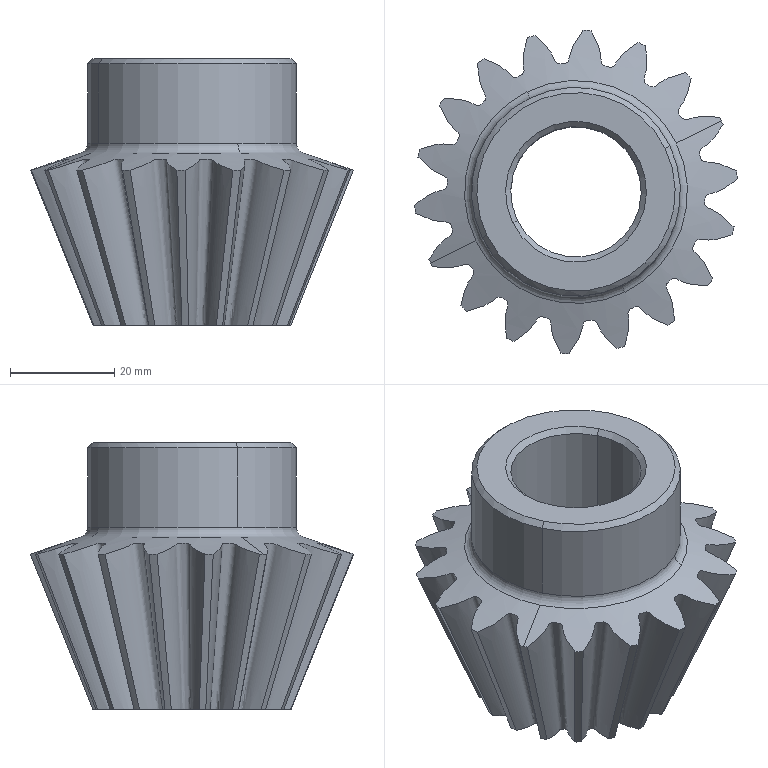Part | SolidWorks | features BaseBody 1 | 1 solid | 51 faces | box 61.792 x 61.935 x 51.071 mm | volume 51754 mm3 | cone 25 | spline 18 | cylinder 4 | torus 2 | plane 2 | commonest cylinder face diameters 25 x2 40 x2